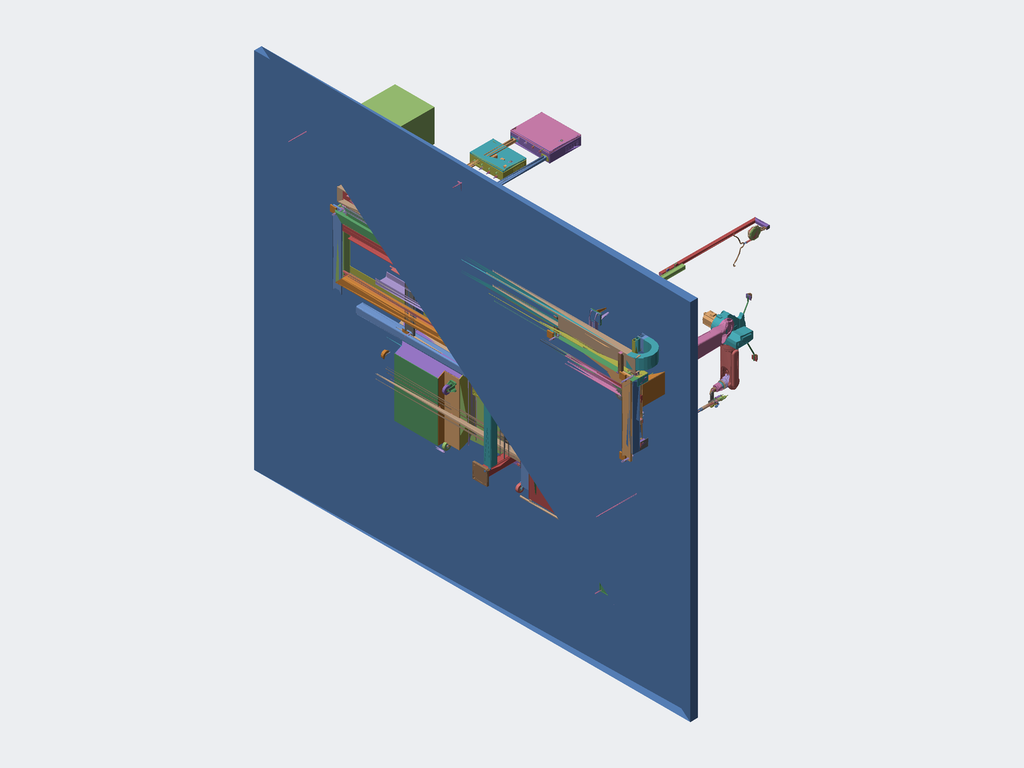Assembly | STEP file | 207 different items | 934 placed
Parts list (item | name | quantity | parent item | size | volume):
1 | 2 fen male thread×8mm | x3 | in HXGR200008-06-02 | 17.321 x 15 x 30.3 mm | 1537 mm3
2 | - | x4 | in Added insulation kit modification | - | -
3 | - | x8 | in Added insulation kit modification | - | -
4 | - | x2 | in Added insulation kit modification | - | -
5 | 20C | x22 | in HXGR200008-06-02, HXGR200008-06-03 | 36 x 13 x 13 mm | 1696 mm3
6 | 2·Ö-8mm | x6 | in HXGR200008-06-02 | - | -
7 | 300221050#MCT225-08 | x1 | in MCT318 (8mm connector) | 74 x 40.976 x 18 mm | 15654 mm3
8 | - | x2 | in MCT318 (8mm connector) | - | -
9 | 300621470#NBM1615L-C | x1 | in MCT318 (8mm connector) | 14 x 19 x 20.5 mm | 1899 mm3
10 | 307 series cutting nozzle | x1 | in HXGR200008-05-22 | - | -
11 | 45C.125.150-42-45C.125.12PZ | x1 | in HXGR200008-05 | 153 x 367 x 2542 mm | 13515724 mm3
12 | 780.0885.0+780.H027.0+780.0512.1+780.0029 | x1 | in HXGR200008-05-22 | 85.965 x 148.6 x 231 mm | 538437 mm3
13 | 7C | x11 | in HXGR200008-06-02, HXGR200008-06-03 | 14 x 19 x 20.5 mm | 1922 mm3
14 | 853PLF-80-N | x1 | in HXGR200008-06-02 | 95 x 117.594 x 66.785 mm | 220085 mm3
15 | 853PLX-200-N | x2 | in HXGR200008-06-02 | 95 x 117.594 x 66.785 mm | 220085 mm3
16 | 8C | x11 | in HXGR200008-06-02, HXGR200008-06-03 | 14 x 19 x 20.5 mm | 1899 mm3
17 | 8mm connector | x3 | in MCT318 (8mm connector) | - | -
18 | A22NE-A-401 | x2 | in HXGR_CZH_DGD_100_HD | 25 x 9 x 25 mm | 2109 mm3
19 | A22NE_M_N_BASE | x1 | in A22NE_M_N | 40 x 40 x 54 mm | 28199 mm3
20 | A22NE_M_N_NUT | x1 | in A22NE_M_N | 29 x 29 x 7.7 mm | 1960 mm3
21 | A22NK_2BM_01AA_G102 | x1 | in HXGR_CZH_DGD_100_HD | 30 x 53 x 88.3 mm | 39098 mm3
22 | A22NL_BGM_TGA_G100_GC | x2 | in HXGR_CZH_DGD_100_HD | 30 x 53 x 64.4 mm | 41405 mm3
23 | A22NN_BMM_NGA_G100_NN | x2 | in HXGR_CZH_DGD_100_HD | 40 x 53 x 66 mm | 35883 mm3
24 | A22NN_BNM_NBA_G100_NN | x1 | in HXGR_CZH_DGD_100_HD | 30 x 53 x 56.3 mm | 27846 mm3
25 | A22NN_BNM_NRA_G100_NN | x1 | in HXGR_CZH_DGD_100_HD | 30 x 53 x 56.3 mm | 27846 mm3
26 | A22NN_BNM_NYA_G100_NN | x1 | in HXGR_CZH_DGD_100_HD | 30 x 53 x 56.3 mm | 27846 mm3
27 | A22NZ-A-301 | x1 | in HXGR_CZH_DGD_100_HD | 20 x 60 x 20 mm | 3581 mm3
28 | A22NZ-A-302 | x1 | in HXGR_CZH_DGD_100_HD | 20 x 60 x 20 mm | 3581 mm3
29 | A22NZ-A-403 | x1 | in 164 | 28.8 x 28.8 x 5 mm | 1033 mm3
30 | A22NZ_2B[]_N[]A_BASE | x1 | in A22NZ_2BM_NBA | 28.8 x 28.8 x 47.2 mm | 14426 mm3
31 | A22NZ_2B[]_N[]A_NUT | x1 | in A22NZ_2BM_NBA | 29 x 29 x 6.8 mm | 1476 mm3
32 | A22NZ_H_01 | x1 | in A22NS_2B[]_N[]A_G00[]_NN_TERMINAL | 30 x 51.298 x 17.1 mm | 5961 mm3
33 | A22NZ_H_01_LEVER | x1 | in A22NS_2B[]_N[]A_G00[]_NN_TERMINAL | 25.4 x 42.2 x 8.2 mm | 1285 mm3
34 | A22NZ_H_02 | x1 | in A22NE_M_P202_N_TERMINAL | 30 x 51.298 x 17.1 mm | 5133 mm3
35 | A22NZ_H_02_LEVER | x1 | in A22NE_M_P202_N_TERMINAL | 25.4 x 42.2 x 10 mm | 1414 mm3
36 | A22NZ_S_G1[] | x1 | in A22NS_2B[]_N[]A_G00[]_NN_TERMINAL | 9.9 x 47 x 29.6 mm | 7656 mm3
37 | A22NZ_S_P1[]N | x2 | in A22NE_M_P202_N_TERMINAL | 9.9 x 47.6 x 23.8 mm | 5482 mm3
38 | A7PH_206_BASE | x2 | in A7PH_206_2UNIT | 14.5 x 33 x 50.2 mm | 11412 mm3
39 | A7P_M_LEFT | x1 | in A7PH_206_2UNIT | 8.8 x 39 x 36.5 mm | 5217 mm3
40 | A7P_M_RIGHT | x1 | in A7PH_206_2UNIT | 13.3 x 39 x 36.5 mm | 5293 mm3
41 | AE hinge | x4 | in Lockable cabinet 460×320×125, Lockable cabinet 540×430×130 | - | -
42 | AG12-6.5 | x4 | in HXGR200008-06-03 | 35 x 18.8 x 18.8 mm | 5027 mm3
43 | ANFX-P130W-1SL3-21 | x1 | in HXGR200008-05-12 | 236 x 122 x 120 mm | 1055212 mm3
44 | Body | x2 | in FA9TO | - | -
45 | Body_1 | x1 | in FA9TF | - | -
46 | CF881.03.25 | x1 | in HXGR_CZH_DGD_100_HD | 11.5 x 11.5 x 500 mm | 51934 mm3
47 | - | x8 | in HXGR200008-06, HXGR_CZH_DGD_100_HD | 20 x 137 x 20 mm | 11527 mm3
48 | - | x10 | in HXGR200008-05 | 30 x 169 x 30 mm | 37532 mm3
49 | DH24-32 | x1 | in HXGR200008-05 | 45 x 276.598 x 178 mm | 145916 mm3
50 | - | x1 | in HXGR_CZH_DGD_100_HD | - | -
51 | EW-3 | x1 | in HXGR200008-05-20 | 149.256 x 72.65 x 284.25 mm | 626000 mm3
52 | Filler block | x1 | in MCT318 (8mm connector) | - | -
53 | - | x1 | in HXGR200008-06-02 | - | -
54 | - | x2 | in HXGR200008-06-02 | - | -
55 | GBT 5781#Hex head bolt fully threaded_M12×100-zinc plated | x4 | in Added insulation kit modification | 107.5 x 20.785 x 18 mm | 13373 mm3
56 | GBT 6170#Type 1 hex nut_M12-steel | x4 | in Added insulation kit modification | - | -
57 | GBT 95#Flat washer_12-zinc plated | x8 | in Added insulation kit modification | - | -
58 | - | x2 | in HXGR200008-05 | 5 x 20 x 5 mm | 390.082 mm3
59 | - | x3 | in HXGR200008-05 | 10 x 70 x 10 mm | 5144 mm3
60 | - | x2 | in HXGR200008-05 | 12 x 55 x 12 mm | 5770 mm3
61 | - | x2 | in HXGR200008-05 | 8 x 35 x 8 mm | 1570 mm3
62 | - | x2 | in HXGR200008-05 | 8 x 40 x 8 mm | 1821 mm3
63 | - | x1 | in HXGR200008-05 | 16 x 8.4 x 18.475 mm | 1391 mm3
64 | - | x10 | in HXGR200008-05 | 30 x 18 x 34.641 mm | 9743 mm3
65 | - | x16 | in HXGR200008-06-03 | 8 x 4.7 x 9.238 mm | 196.298 mm3
66 | - | x8 | in HXGR200008-05 | 10 x 5.2 x 11.547 mm | 349.391 mm3
67 | - | x2 | in HXGR200008-05 | 13 x 6.8 x 15.011 mm | 754.504 mm3
68 | - | x4 | in HXGR200008-05 | 16 x 30 x 16 mm | 3301 mm3
69 | - | x5 | in HXGR200008-05, HXGR200008-05-12 | 16 x 35 x 16 mm | 3694 mm3
70 | - | x4 | in HXGR200008-05 | 16 x 40 x 16 mm | 4087 mm3
71 | - | x1 | in HXGR200008-05 | 16 x 75 x 16 mm | 6836 mm3
72 | - | x16 | in HXGR200008-05 | 18 x 47 x 18 mm | 6485 mm3
73 | - | x4 | in HXGR200008-05 | 18 x 62 x 18 mm | 8181 mm3
74 | - | x4 | in HXGR200008-05 | 24 x 71 x 24 mm | 16928 mm3
75 | - | x10 | in HXGR200008-05 | 30 x 90 x 30 mm | 33602 mm3
76 | - | x28 | in HXGR200008-06, HXGR200008-06-03 | 8.5 x 15 x 8.5 mm | 445.038 mm3
77 | - | x8 | in HXGR200008-05 | 8.5 x 13 x 8.5 mm | 405.768 mm3
78 | - | x8 | in HXGR200008-06 | 10 x 16 x 10 mm | 688.299 mm3
79 | - | x8 | in HXGR200008-05 | 10 x 18 x 10 mm | 744.847 mm3
80 | - | x18 | in HXGR200008-05 | 10 x 22 x 10 mm | 857.945 mm3
81 | - | x4 | in HXGR200008-05 | 10 x 26 x 10 mm | 971.042 mm3
82 | - | x6 | in HXGR200008-05 | 10 x 36 x 10 mm | 1254 mm3
83 | - | x4 | in HXGR200008-05-20 | 13 x 24 x 13 mm | 1739 mm3
84 | - | x4 | in HXGR200008-05 | 13 x 28 x 13 mm | 1940 mm3
85 | - | x8 | in HXGR200008-05 | 13 x 33 x 13 mm | 2191 mm3
86 | - | x120 | in HXGR200008-05, HXGR200008-05-12 | 13 x 43 x 13 mm | 2694 mm3
87 | - | x4 | in HXGR200008-05 | 13 x 48 x 13 mm | 2945 mm3
88 | - | x37 | in HXGR200008-05 | 13 x 53 x 13 mm | 3197 mm3
89 | - | x2 | in HXGR200008-05 | 13 x 63 x 13 mm | 3699 mm3
90 | - | x4 | in HXGR200008-05-12 | 13 x 68 x 13 mm | 3951 mm3
91 | - | x17 | in HXGR200008-06-02, HXGR_CZH_DGD_100_HD | 7 x 12.378 x 7 mm | 131.512 mm3
92 | - | x4 | in HXGR_CZH_DGD_100_HD | 10 x 15.681 x 10 mm | 491.081 mm3
93 | - | x48 | in HXGR200008-05 | 12 x 20.569 x 12 mm | 958.317 mm3
94 | - | x1 | in HXGR200008-05-12 | 20 x 2 x 20 mm | 455.138 mm3
95 | - | x4 | in HXGR200008-05 | 24 x 2.5 x 24 mm | 799.143 mm3
96 | - | x4 | in HXGR200008-05-12 | 16 x 1.6 x 16 mm | 233.031 mm3
97 | Gas robot platform[1] | x1 | in JQR-01 | - | -
98 | Grip tube | x1 | in MCT318 (8mm connector) | - | -
99 | Ground | x1 | in JQR-01 | - | -
100 | H06-01S | x8 | in HXGR200008-05 | 13.856 x 24.2 x 12 mm | 1991 mm3
101 | - | x1 | in HXGR200008-05 | - | -
102 | HXGR200008-05-02 | x4 | in HXGR200008-05 | 50 x 73 x 30 mm | 90409 mm3
103 | HXGR200008-05-03 | x4 | in HXGR200008-05 | 25 x 25 x 30 mm | 11121 mm3
104 | HXGR200008-05-04 | x2 | in HXGR200008-05 | 98 x 150 x 2052 mm | 1030227 mm3
105 | HXGR200008-05-04R | x2 | in HXGR200008-05 | 98 x 150 x 2052 mm | 1030227 mm3
106 | HXGR200008-05-05 | x1 | in HXGR200008-05 | 874 x 32 x 800 mm | 19833550 mm3
107 | HXGR200008-05-06 | x1 | in HXGR200008-05 | 150 x 25 x 25 mm | 82216 mm3
108 | HXGR200008-05-07 | x2 | in HXGR200008-05 | 70 x 30 x 25 mm | 44261 mm3
109 | HXGR200008-05-08 | x1 | in HXGR200008-05 | 100 x 60 x 40 mm | 99565 mm3
110 | HXGR200008-05-09 | x1 | in HXGR200008-05 | 40 x 42 x 20 mm | 28088 mm3
111 | HXGR200008-05-10 | x2 | in HXGR200008-05 | 180 x 80 x 2050 mm | 1362117 mm3
112 | HXGR200008-05-11 | x4 | in HXGR200008-05 | 200 x 48 x 100 mm | 720235 mm3
113 | HXGR200008-05-12-01 | x1 | in HXGR200008-05-12 | 200 x 25 x 160 mm | 486660 mm3
114 | HXGR200008-05-12-02 | x1 | in HXGR200008-05-12 | 48 x 48 x 6 mm | 10179 mm3
115 | HXGR200008-05-12-03 | x1 | in HXGR200008-05-12 | 32 x 32 x 85 mm | 43804 mm3
116 | HXGR200008-05-12-04 | x1 | in HXGR200008-05-12 | 120 x 120 x 36 mm | 216881 mm3
117 | - | x1 | in HXGR200008-05 | - | -
118 | HXGR200008-05-14 | x1 | in HXGR200008-05 | 270 x 375 x 331 mm | 959853 mm3
119 | HXGR200008-05-15 | x2 | in HXGR200008-05 | 60 x 30 x 3 mm | 5141 mm3
120 | HXGR200008-05-16 | x2 | in HXGR200008-05 | 187 x 12 x 1000 mm | 408850 mm3
121 | - | x6 | in HXGR200008-05 | - | -
122 | HXGR200008-05-18 | x3 | in HXGR200008-05 | 70 x 42 x 1210 mm | 257088 mm3
123 | - | x1 | in HXGR200008-05 | - | -
124 | HXGR200008-05-20-01 | x1 | in HXGR200008-05-20 | 140 x 140 x 1208 mm | 946089 mm3
125 | - | x1 | in HXGR200008-05-20 | - | -
126 | HXGR200008-05-20-03 | x1 | in HXGR200008-05-20 | 408 x 150 x 8 mm | 28410 mm3
127 | - | x1 | in HXGR200008-05 | - | -
128 | HXGR200008-05-22-05 | x1 | in HXGR200008-05-22 | 43 x 48 x 47.995 mm | 16067 mm3
129 | HXGR200008-05-23 | x1 | in HXGR200008-05 | 65 x 818.205 x 225 mm | 155095 mm3
130 | HXGR200008-05-24 | x2 | in HXGR200008-05 | 65 x 32.5 x 50 mm | 5278 mm3
131 | - | x1 | in HXGR200008-05 | - | -
132 | HXGR200008-05-26 | x1 | in HXGR200008-05 | 50 x 100 x 50 mm | 49486 mm3
133 | HXGR200008-05-27 | x10 | in HXGR200008-05 | 80 x 16 x 80 mm | 101387 mm3
134 | - | x1 | in HXGR200008-06 | - | -
135 | HXGR200008-06-02-01 | x3 | in HXGR200008-06-02 | 46 x 46 x 2 mm | 1252 mm3
136 | HXGR200008-06-02-02 | x1 | in HXGR200008-06-02 | 55 x 15 x 1 mm | 818.886 mm3
137 | HXGR200008-06-02-03 | x1 | in HXGR200008-06-02 | 55 x 15 x 1 mm | 815.181 mm3
138 | HXGR200008-06-02-04 | x1 | in HXGR200008-06-02 | 55 x 15 x 1 mm | 821.434 mm3
139 | HXGR200008-06-02-05 | x1 | in HXGR200008-06-02 | 55 x 15 x 1 mm | 817.796 mm3
140 | HXGR200008-06-02-06 | x1 | in HXGR200008-06-02 | 55 x 15 x 1 mm | 818.976 mm3
141 | HXGR200008-06-02-07 | x1 | in HXGR200008-06-02 | 55 x 15 x 1 mm | 815.332 mm3
142 | HXGR200008-06-02-08 | x3 | in HXGR200008-06-02 | 55 x 15 x 1 mm | 774.16 mm3
143 | HXGR200008-06-03-01 | x4 | in HXGR200008-06-03 | 35 x 15.5 x 72 mm | 6389 mm3
144 | HXGR200008-06-03-02 | x4 | in HXGR200008-06-03 | 22 x 20 x 31.6 mm | 6606 mm3
145 | HXGR200008-06-03-03 | x4 | in HXGR200008-06-03 | 22 x 20 x 31.6 mm | 6624 mm3
146 | HXGR200008-06-03-04_M16 | x7 | in HXGR200008-06-02, HXGR200008-06-03 | 24 x 27.713 x 8 mm | 2454 mm3
147 | HXGR200008-06-03-05 | x7 | in HXGR200008-06-02, HXGR200008-06-03 | 16 x 56 x 22 mm | 5972 mm3
148 | HXGR200008-06-03-06_M16 | x7 | in HXGR200008-06-02, HXGR200008-06-03 | 24 x 27.713 x 8 mm | 2461 mm3
149 | HXGR200008-06-03-07 | x7 | in HXGR200008-06-02, HXGR200008-06-03 | 16 x 56 x 22 mm | 5981 mm3
150 | HXGR200008-07 | x1 | in JQR-01 | 700 x 165 x 580 mm | 3623561 mm3
151 | Inner sleeve | x2 | in FA9TO | - | -
152 | Inner sleeve_1 | x1 | in FA9TF | - | -
153 | - | x4 | in HXGR200008-05 | 11 x 18 x 12.702 mm | 898.198 mm3
154 | Link1 | x1 | in NV25 | 539 x 508 x 522 mm | 37862681 mm3
155 | Link1_mot | x1 | in NV25 | 130 x 220 x 147 mm | 2850182 mm3
156 | Link2 | x1 | in NV25 | 1001 x 272 x 134 mm | 13121493 mm3
157 | Link3 | x1 | in NV25 | 424.142 x 365 x 328.5 mm | 12864822 mm3
158 | Link3_J3mot | x1 | in NV25 | 130 x 147 x 155 mm | 2279615 mm3
159 | Link3_J4mot | x1 | in NV25 | 94.4 x 124 x 80 mm | 690172 mm3
160 | Link4 | x1 | in NV25 | 228 x 227 x 571.1 mm | 9720047 mm3
161 | Link5 | x1 | in NV25 | 130 x 161.5 x 98 mm | 1253292 mm3
162 | Link6 | x1 | in NV25 | 98 x 96.836 x 18 mm | 95263 mm3
163 | - | x3 | in HXGR200008-06-02 | 45.215 x 17 x 41.128 mm | 7498 mm3
164 | M22N-BG-TGA-GC | x1 | in 164 | 30 x 29.9 x 64.7 mm | 28524 mm3
165 | M8C | x100 | in HXGR200008-05 | 14 x 14 x 4 mm | 606.615 mm3
166 | MH042640 | x1 | in HXGR200008-05-12 | - | -
167 | MHH043906 | x1 | in HXGR200008-05 | 613.8 x 39 x 39 mm | 892867 mm3
168 | MHH043910 | x3 | in HXGR200008-05 | 1014 x 39 x 39 mm | 1489427 mm3
169 | - | x4 | in MS705[ MS705]_ MS705 | 18.6 x 1.8 x 18.6 mm | 134.306 mm3
170 | - | x2 | in MS705[ MS705]_ MS705 | 17.57 x 17.57 x 0.8 mm | 124.693 mm3
171 | Nozzle | x2 | in FA9TO | - | -
172 | Nozzle_1 | x1 | in FA9TF | - | -
173 | Nut left-hand | x1 | in FA9TF | - | -
174 | Nut right-hand | x2 | in FA9TO | - | -
175 | OL-A | x4 | in HXGR200008-05 | 12 x 23.5 x 12 mm | 1623 mm3
176 | PD19 | x1 | in JQR-01 | 542 x 640 x 441 mm | 152648654 mm3
177 | PN_0013_Default<As machined> | x1 | in HXGR_CZH_DGD_100_HD | - | -
178 | PN_0014_Default<As machined> | x1 | in HXGR_CZH_DGD_100_HD | - | -
179 | PN_0023[ PN_0023]_Base_Base | x2 | in MS705[ MS705]_ MS705 | - | -
180 | PN_0023[ PN_0023]_Door panel_Door panel | x2 | in MS705[ MS705]_ MS705 | - | -
181 | PN_0023[ PN_0023]_GB/T 808-1988 small hex thin nut M22×1(A3)_Nut M22×1 | x2 | in MS705[ MS705]_ MS705 | 27 x 31.177 x 3.74 mm | 939.292 mm3
182 | PN_0023[ PN_0023]_Lock cylinder_triangle 8mm | x2 | in MS705[ MS705]_ MS705 | - | -
183 | PN_0023[ PN_0023]_PN_0024 steel bolt_PN_0023 steel bolt | x2 | in MS705[ MS705]_ MS705 | - | -
184 | PN_0023[ PN_0023]_Screw_Screw | x2 | in MS705[ MS705]_ MS705 | - | -
185 | PN_0023[ PN_0023]_Sealing gasket_Sealing gasket | x2 | in MS705[ MS705]_ MS705 | - | -
186 | Regulator box body_Default<As machined> | x1 | in Lockable cabinet 540×430×130 | - | -
187 | Regulator box cover | x1 | in Lockable cabinet 540×430×130 | - | -
188 | Solenoid valve housing box body_Default<As machined> | x1 | in Lockable cabinet 460×320×125 | - | -
189 | Solenoid valve housing box lid | x1 | in Lockable cabinet 460×320×125 | - | -
190 | Steel tube | x3 | in MCT318 (8mm connector) | - | -
191 | W-L02641 | x1 | in HXGR200008-05-12 | 130 x 147 x 190 mm | 2320487 mm3
192 | WS28J26TQ_SW28 | x2 | in HXGR_CZH_DGD_100_HD | 33.799 x 33.799 x 68.56 mm | 40165 mm3
193 | WS28K26Z | x2 | in HXGR_CZH_DGD_100_HD | 36 x 36 x 27 mm | 15562 mm3
194 | _2W050-10 - Valve Body_3 | x4 | in 2W05010B | 31 x 33.1 x 52 mm | 37605 mm3
195 | _2W050-15 - Valve Terminal_3 | x4 | in 2W05010B | 39 x 55.5 x 86.1 mm | 126239 mm3
196 | _MSA35A2SS+R3980-30_30N2_(G-M61SSG-M6) | x2 | - | 3980 x 29 x 34 mm | 3160626 mm3
197 | _MSA35ES | x8 | - | 3.6 x 36.3 x 67.6 mm | 6318 mm3
198 | _MSA35ESSFCN | x4 | - | 104 x 38.5 x 100 mm | 261155 mm3
199 | base | x1 | in NV25 | 518 x 391 x 191.5 mm | 24353217 mm3
200 | - | x1 | in MCT318 (8mm connector) | - | -
201 | - | x2 | in MCT318 (8mm connector) | - | -
202 | - | x1 | in MCT318 (8mm connector) | - | -
203 | - | x1 | in MCT318 (8mm connector) | - | -
204 | - | x2 | in MCT318 (8mm connector) | - | -
205 | - | x1 | in MCT318 (8mm connector) | - | -
206 | - | x1 | in MCT318 (8mm connector) | - | -
207 | - | x3 | in MCT318 (8mm connector) | - | -